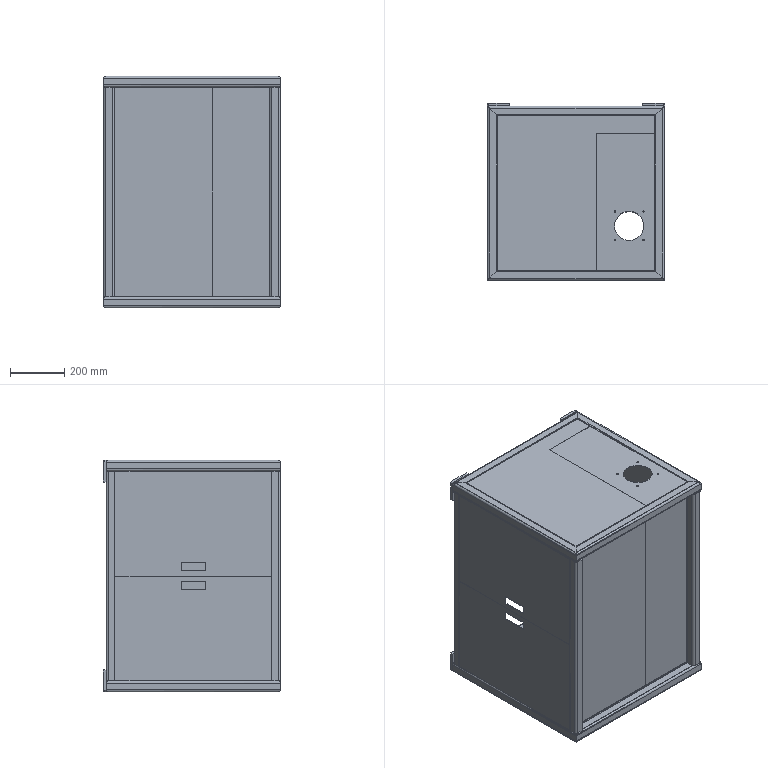Part | STEP file | Frame_default<machined> | 21 solids | 390 faces | box 650 x 650 x 850 mm | volume 14326768 mm3 | plane 222 | cylinder 168 | commonest cylinder face diameters 5 x56 16 x50 8 x48 40 x8 107 x4 15 x2